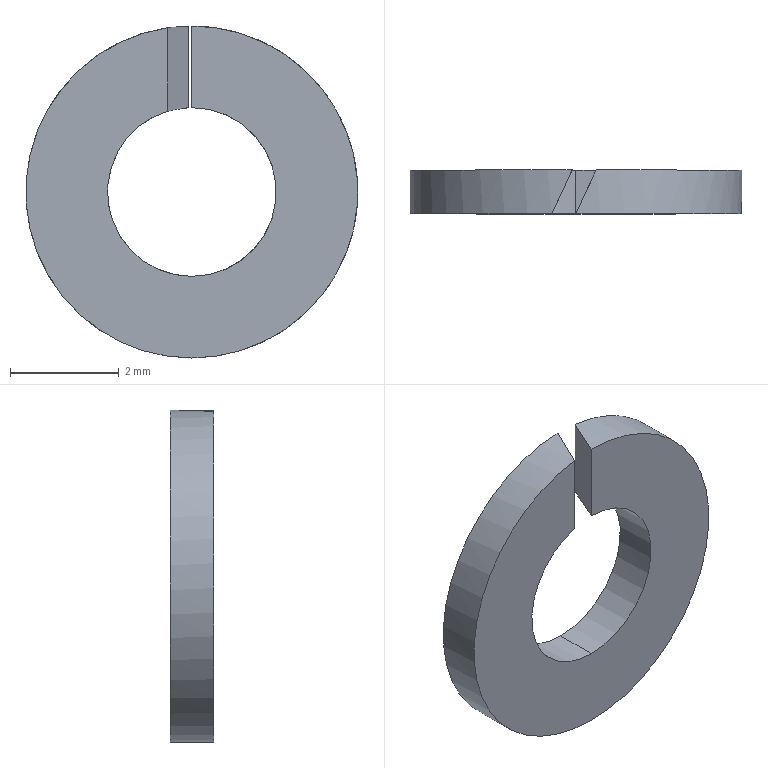Part | SolidWorks | features Extrusion 1, ICE 1, RefAxis 1 | 1 solid | 8 faces | box 6.1 x 0.8 x 6.1 mm | volume 16.81 mm3 | cylinder 4 | plane 4 | commonest cylinder face diameters 3.1 x2 6.1 x2
STEP:
#1=CARTESIAN_POINT('',(0.373,0.8,1.504));
#2=VERTEX_POINT('',#1);
#3=CARTESIAN_POINT('',(0.,0.8,-1.55));
#4=VERTEX_POINT('',#3);
#5=CARTESIAN_POINT('',(0.,0.8,0.));
#6=DIRECTION('',(0.,1.,0.));
#7=DIRECTION('',(0.,0.,1.));
#8=AXIS2_PLACEMENT_3D('',#5,#6,#7);
#9=CIRCLE('',#8,1.55);
#10=EDGE_CURVE('',#2,#4,#9,.T.);
#11=ORIENTED_EDGE('',*,*,#10,.T.);
#12=CARTESIAN_POINT('',(0.,0.,-1.55));
#13=VERTEX_POINT('',#12);
#14=CARTESIAN_POINT('',(0.,0.8,-1.55));
#15=DIRECTION('',(0.,-1.,0.));
#16=VECTOR('',#15,1000.);
#17=LINE('',#14,#16);
#18=EDGE_CURVE('',#4,#13,#17,.T.);
#19=ORIENTED_EDGE('',*,*,#18,.T.);
#20=CARTESIAN_POINT('',(0.,0.,1.55));
#21=VERTEX_POINT('',#20);
#22=CARTESIAN_POINT('',(0.,0.,0.));
#23=DIRECTION('',(0.,1.,0.));
#24=DIRECTION('',(0.,0.,1.));
#25=AXIS2_PLACEMENT_3D('',#22,#23,#24);
#26=CIRCLE('',#25,1.55);
#27=EDGE_CURVE('',#21,#13,#26,.T.);
#28=ORIENTED_EDGE('',*,*,#27,.F.);
#29=CARTESIAN_POINT('',(0.,0.,1.55));
#30=CARTESIAN_POINT('',(0.1259,0.27,1.55));
#31=CARTESIAN_POINT('',(0.2509,0.538,1.535));
#32=CARTESIAN_POINT('',(0.373,0.8,1.504));
#33=(BOUNDED_CURVE()B_SPLINE_CURVE(3,(#29,#30,#31,#32),.UNSPECIFIED.,.F.,.F.)B_SPLINE_CURVE_WITH_KNOTS((4,4),(1.571,1.814),.UNSPECIFIED.)CURVE()GEOMETRIC_REPRESENTATION_ITEM()RATIONAL_B_SPLINE_CURVE((1.,0.9951,0.9951,1.))REPRESENTATION_ITEM(''));
#34=EDGE_CURVE('',#21,#2,#33,.T.);
#35=ORIENTED_EDGE('',*,*,#34,.T.);
#36=EDGE_LOOP('',(#11,#19,#28,#35));
#37=FACE_OUTER_BOUND('',#36,.T.);
#38=CARTESIAN_POINT('',(0.,0.8,0.));
#39=DIRECTION('',(0.,-1.,0.));
#40=DIRECTION('',(0.,0.,-1.));
#41=AXIS2_PLACEMENT_3D('',#38,#39,#40);
#42=CYLINDRICAL_SURFACE('',#41,1.55);
#43=ADVANCED_FACE('',(#37),#42,.F.);
#44=CARTESIAN_POINT('',(0.,0.8,-3.05));
#45=VERTEX_POINT('',#44);
#46=CARTESIAN_POINT('',(-0.06831,0.8,3.049));
#47=VERTEX_POINT('',#46);
#48=CARTESIAN_POINT('',(0.,0.8,0.));
#49=DIRECTION('',(0.,1.,0.));
#50=DIRECTION('',(0.,0.,1.));
#51=AXIS2_PLACEMENT_3D('',#48,#49,#50);
#52=CIRCLE('',#51,3.05);
#53=EDGE_CURVE('',#45,#47,#52,.T.);
#54=ORIENTED_EDGE('',*,*,#53,.F.);
#55=CARTESIAN_POINT('',(0.,0.,-3.05));
#56=VERTEX_POINT('',#55);
#57=CARTESIAN_POINT('',(0.,0.8,-3.05));
#58=DIRECTION('',(0.,-1.,0.));
#59=VECTOR('',#58,1000.);
#60=LINE('',#57,#59);
#61=EDGE_CURVE('',#45,#56,#60,.T.);
#62=ORIENTED_EDGE('',*,*,#61,.T.);
#63=CARTESIAN_POINT('',(-0.4414,0.,3.018));
#64=VERTEX_POINT('',#63);
#65=CARTESIAN_POINT('',(0.,0.,0.));
#66=DIRECTION('',(0.,1.,0.));
#67=DIRECTION('',(0.,0.,1.));
#68=AXIS2_PLACEMENT_3D('',#65,#66,#67);
#69=CIRCLE('',#68,3.05);
#70=EDGE_CURVE('',#56,#64,#69,.T.);
#71=ORIENTED_EDGE('',*,*,#70,.T.);
#72=CARTESIAN_POINT('',(-0.06831,0.8,3.049));
#73=CARTESIAN_POINT('',(-0.1932,0.5321,3.046));
#74=CARTESIAN_POINT('',(-0.3177,0.2651,3.036));
#75=CARTESIAN_POINT('',(-0.4414,0.,3.018));
#76=(BOUNDED_CURVE()B_SPLINE_CURVE(3,(#72,#73,#74,#75),.UNSPECIFIED.,.F.,.T.)B_SPLINE_CURVE_WITH_KNOTS((4,4),(4.735,4.858),.UNSPECIFIED.)CURVE()GEOMETRIC_REPRESENTATION_ITEM()RATIONAL_B_SPLINE_CURVE((1.,0.9987,0.9987,1.))REPRESENTATION_ITEM(''));
#77=EDGE_CURVE('',#47,#64,#76,.T.);
#78=ORIENTED_EDGE('',*,*,#77,.F.);
#79=EDGE_LOOP('',(#54,#62,#71,#78));
#80=FACE_OUTER_BOUND('',#79,.T.);
#81=CARTESIAN_POINT('',(0.,0.8,0.));
#82=DIRECTION('',(0.,-1.,0.));
#83=DIRECTION('',(0.,0.,-1.));
#84=AXIS2_PLACEMENT_3D('',#81,#82,#83);
#85=CYLINDRICAL_SURFACE('',#84,3.05);
#86=ADVANCED_FACE('',(#80),#85,.T.);
#87=ORIENTED_EDGE('',*,*,#10,.F.);
#88=CARTESIAN_POINT('',(0.373,0.8,3.027));
#89=VERTEX_POINT('',#88);
#90=CARTESIAN_POINT('',(0.373,0.8,3.05));
#91=DIRECTION('',(0.,0.,-1.));
#92=VECTOR('',#91,1000.);
#93=LINE('',#90,#92);
#94=EDGE_CURVE('',#89,#2,#93,.T.);
#95=ORIENTED_EDGE('',*,*,#94,.F.);
#96=CARTESIAN_POINT('',(0.,0.8,0.));
#97=DIRECTION('',(0.,1.,0.));
#98=DIRECTION('',(0.,0.,1.));
#99=AXIS2_PLACEMENT_3D('',#96,#97,#98);
#100=CIRCLE('',#99,3.05);
#101=EDGE_CURVE('',#89,#45,#100,.T.);
#102=ORIENTED_EDGE('',*,*,#101,.T.);
#103=ORIENTED_EDGE('',*,*,#53,.T.);
#104=CARTESIAN_POINT('',(-0.06831,0.8,1.548));
#105=VERTEX_POINT('',#104);
#106=CARTESIAN_POINT('',(-0.06831,0.8,3.05));
#107=DIRECTION('',(0.,0.,-1.));
#108=VECTOR('',#107,1000.);
#109=LINE('',#106,#108);
#110=EDGE_CURVE('',#47,#105,#109,.T.);
#111=ORIENTED_EDGE('',*,*,#110,.T.);
#112=CARTESIAN_POINT('',(0.,0.8,0.));
#113=DIRECTION('',(0.,1.,0.));
#114=DIRECTION('',(0.,0.,1.));
#115=AXIS2_PLACEMENT_3D('',#112,#113,#114);
#116=CIRCLE('',#115,1.55);
#117=EDGE_CURVE('',#4,#105,#116,.T.);
#118=ORIENTED_EDGE('',*,*,#117,.F.);
#119=EDGE_LOOP('',(#87,#95,#102,#103,#111,#118));
#120=FACE_OUTER_BOUND('',#119,.T.);
#121=CARTESIAN_POINT('',(0.,0.8,0.));
#122=DIRECTION('',(0.,1.,0.));
#123=DIRECTION('',(0.,0.,1.));
#124=AXIS2_PLACEMENT_3D('',#121,#122,#123);
#125=PLANE('',#124);
#126=ADVANCED_FACE('',(#120),#125,.T.);
#127=CARTESIAN_POINT('',(0.,0.,3.05));
#128=VERTEX_POINT('',#127);
#129=CARTESIAN_POINT('',(0.,0.,3.05));
#130=DIRECTION('',(0.,0.,-1.));
#131=VECTOR('',#130,1000.);
#132=LINE('',#129,#131);
#133=EDGE_CURVE('',#128,#21,#132,.T.);
#134=ORIENTED_EDGE('',*,*,#133,.T.);
#135=ORIENTED_EDGE('',*,*,#27,.T.);
#136=CARTESIAN_POINT('',(-0.4414,0.,1.486));
#137=VERTEX_POINT('',#136);
#138=CARTESIAN_POINT('',(0.,0.,0.));
#139=DIRECTION('',(0.,1.,0.));
#140=DIRECTION('',(0.,0.,1.));
#141=AXIS2_PLACEMENT_3D('',#138,#139,#140);
#142=CIRCLE('',#141,1.55);
#143=EDGE_CURVE('',#13,#137,#142,.T.);
#144=ORIENTED_EDGE('',*,*,#143,.T.);
#145=CARTESIAN_POINT('',(-0.4414,0.,3.05));
#146=DIRECTION('',(0.,0.,-1.));
#147=VECTOR('',#146,1000.);
#148=LINE('',#145,#147);
#149=EDGE_CURVE('',#64,#137,#148,.T.);
#150=ORIENTED_EDGE('',*,*,#149,.F.);
#151=ORIENTED_EDGE('',*,*,#70,.F.);
#152=CARTESIAN_POINT('',(0.,0.,0.));
#153=DIRECTION('',(0.,1.,0.));
#154=DIRECTION('',(0.,0.,1.));
#155=AXIS2_PLACEMENT_3D('',#152,#153,#154);
#156=CIRCLE('',#155,3.05);
#157=EDGE_CURVE('',#128,#56,#156,.T.);
#158=ORIENTED_EDGE('',*,*,#157,.F.);
#159=EDGE_LOOP('',(#134,#135,#144,#150,#151,#158));
#160=FACE_OUTER_BOUND('',#159,.T.);
#161=CARTESIAN_POINT('',(0.,0.,0.));
#162=DIRECTION('',(0.,1.,0.));
#163=DIRECTION('',(0.,0.,1.));
#164=AXIS2_PLACEMENT_3D('',#161,#162,#163);
#165=PLANE('',#164);
#166=ADVANCED_FACE('',(#160),#165,.F.);
#167=ORIENTED_EDGE('',*,*,#61,.F.);
#168=ORIENTED_EDGE('',*,*,#101,.F.);
#169=CARTESIAN_POINT('',(0.,0.,3.05));
#170=CARTESIAN_POINT('',(0.1247,0.2675,3.05));
#171=CARTESIAN_POINT('',(0.2492,0.5345,3.042));
#172=CARTESIAN_POINT('',(0.373,0.8,3.027));
#173=(BOUNDED_CURVE()B_SPLINE_CURVE(3,(#169,#170,#171,#172),.UNSPECIFIED.,.F.,.F.)B_SPLINE_CURVE_WITH_KNOTS((4,4),(1.571,1.693),.UNSPECIFIED.)CURVE()GEOMETRIC_REPRESENTATION_ITEM()RATIONAL_B_SPLINE_CURVE((1.,0.9987,0.9987,1.))REPRESENTATION_ITEM(''));
#174=EDGE_CURVE('',#128,#89,#173,.T.);
#175=ORIENTED_EDGE('',*,*,#174,.F.);
#176=ORIENTED_EDGE('',*,*,#157,.T.);
#177=EDGE_LOOP('',(#167,#168,#175,#176));
#178=FACE_OUTER_BOUND('',#177,.T.);
#179=CARTESIAN_POINT('',(0.,0.8,0.));
#180=DIRECTION('',(0.,-1.,0.));
#181=DIRECTION('',(0.,0.,-1.));
#182=AXIS2_PLACEMENT_3D('',#179,#180,#181);
#183=CYLINDRICAL_SURFACE('',#182,3.05);
#184=ADVANCED_FACE('',(#178),#183,.T.);
#185=ORIENTED_EDGE('',*,*,#18,.F.);
#186=ORIENTED_EDGE('',*,*,#117,.T.);
#187=CARTESIAN_POINT('',(-0.06831,0.8,1.548));
#188=CARTESIAN_POINT('',(-0.1949,0.5285,1.543));
#189=CARTESIAN_POINT('',(-0.3199,0.2605,1.522));
#190=CARTESIAN_POINT('',(-0.4414,0.,1.486));
#191=(BOUNDED_CURVE()B_SPLINE_CURVE(3,(#187,#188,#189,#190),.UNSPECIFIED.,.F.,.T.)B_SPLINE_CURVE_WITH_KNOTS((4,4),(4.756,5.001),.UNSPECIFIED.)CURVE()GEOMETRIC_REPRESENTATION_ITEM()RATIONAL_B_SPLINE_CURVE((1.,0.995,0.995,1.))REPRESENTATION_ITEM(''));
#192=EDGE_CURVE('',#105,#137,#191,.T.);
#193=ORIENTED_EDGE('',*,*,#192,.T.);
#194=ORIENTED_EDGE('',*,*,#143,.F.);
#195=EDGE_LOOP('',(#185,#186,#193,#194));
#196=FACE_OUTER_BOUND('',#195,.T.);
#197=CARTESIAN_POINT('',(0.,0.8,0.));
#198=DIRECTION('',(0.,-1.,0.));
#199=DIRECTION('',(0.,0.,-1.));
#200=AXIS2_PLACEMENT_3D('',#197,#198,#199);
#201=CYLINDRICAL_SURFACE('',#200,1.55);
#202=ADVANCED_FACE('',(#196),#201,.F.);
#203=ORIENTED_EDGE('',*,*,#77,.T.);
#204=ORIENTED_EDGE('',*,*,#149,.T.);
#205=ORIENTED_EDGE('',*,*,#192,.F.);
#206=ORIENTED_EDGE('',*,*,#110,.F.);
#207=EDGE_LOOP('',(#203,#204,#205,#206));
#208=FACE_OUTER_BOUND('',#207,.T.);
#209=CARTESIAN_POINT('',(-0.06831,0.8,3.05));
#210=DIRECTION('',(0.9063,-0.4226,0.));
#211=DIRECTION('',(0.4226,0.9063,0.));
#212=AXIS2_PLACEMENT_3D('',#209,#210,#211);
#213=PLANE('',#212);
#214=ADVANCED_FACE('',(#208),#213,.T.);
#215=ORIENTED_EDGE('',*,*,#174,.T.);
#216=ORIENTED_EDGE('',*,*,#94,.T.);
#217=ORIENTED_EDGE('',*,*,#34,.F.);
#218=ORIENTED_EDGE('',*,*,#133,.F.);
#219=EDGE_LOOP('',(#215,#216,#217,#218));
#220=FACE_OUTER_BOUND('',#219,.T.);
#221=CARTESIAN_POINT('',(0.,0.,3.05));
#222=DIRECTION('',(-0.9063,0.4226,0.));
#223=DIRECTION('',(-0.4226,-0.9063,0.));
#224=AXIS2_PLACEMENT_3D('',#221,#222,#223);
#225=PLANE('',#224);
#226=ADVANCED_FACE('',(#220),#225,.T.);
#227=CLOSED_SHELL('',(#43,#86,#126,#166,#184,#202,#214,#226));
#228=MANIFOLD_SOLID_BREP('',#227);
#229=CARTESIAN_POINT('',(0.,0.,0.));
#230=DIRECTION('',(0.,0.,1.));
#231=DIRECTION('',(1.,0.,0.));
#232=AXIS2_PLACEMENT_3D('',#229,#230,#231);
#233=(LENGTH_UNIT()NAMED_UNIT(*)SI_UNIT(.MILLI.,.METRE.));
#234=UNCERTAINTY_MEASURE_WITH_UNIT(LENGTH_MEASURE(0.00001),#233,'','');
#235=(NAMED_UNIT(*)PLANE_ANGLE_UNIT()SI_UNIT($,.RADIAN.));
#236=(NAMED_UNIT(*)SI_UNIT($,.STERADIAN.)SOLID_ANGLE_UNIT());
#237=(GEOMETRIC_REPRESENTATION_CONTEXT(3)GLOBAL_UNCERTAINTY_ASSIGNED_CONTEXT((#234))GLOBAL_UNIT_ASSIGNED_CONTEXT((#233,#235,#236))REPRESENTATION_CONTEXT('',''));
#238=ADVANCED_BREP_SHAPE_REPRESENTATION('',(#228,#232),#237);